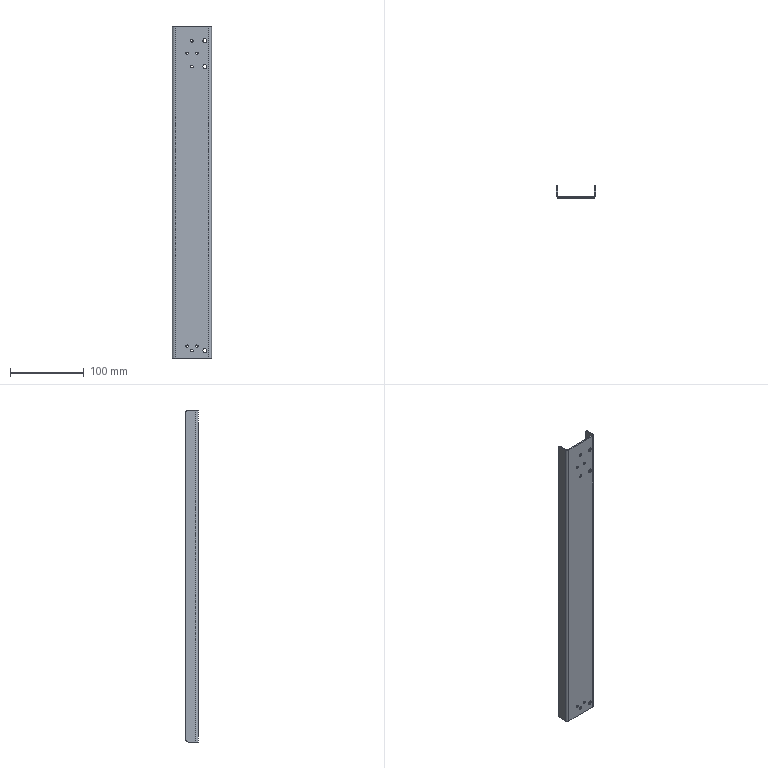Part | STEP file | 0-19-21 Drag chain support plate | 1 solid | 46 faces | box 53 x 16.5 x 450 mm | volume 54218 mm3 | cylinder 28 | plane 18 | commonest cylinder face diameters 3.3 x8 3.5 x6 5.5 x6 6 x4 4 x2 7 x2